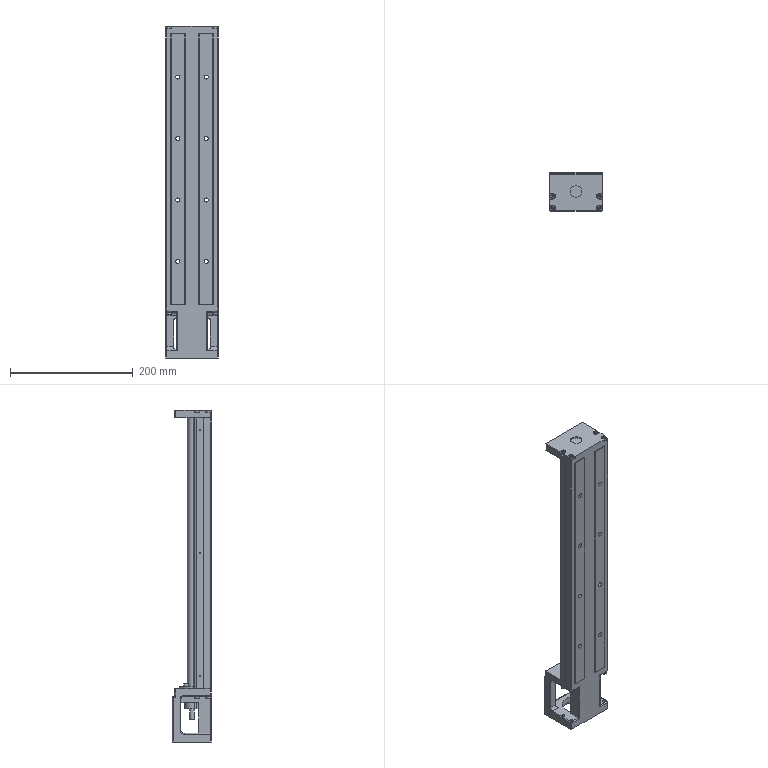Part | NX | 1 solid | 357 faces | box 86 x 64 x 540 mm | volume 926769 mm3 | plane 218 | cylinder 116 | spline 14 | cone 9 | commonest cylinder face diameters 3 x31 6 x12 7.5 x12 3.3 x8 4.5 x8 6.6 x8